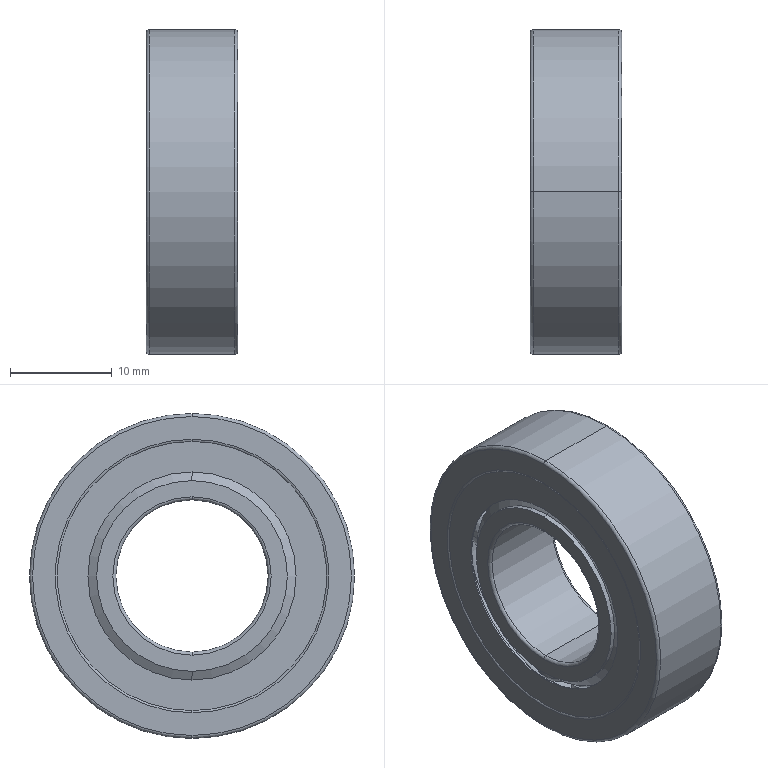Part | SolidWorks | features Revolution 5, CirPattern 2, RefAxis 1, RevCut 1 | 16 solids | 192 faces | box 9 x 32 x 32 mm | volume 4173 mm3 | cylinder 70 | sphere 60 | plane 36 | torus 22 | cone 4 | commonest cylinder face diameters 22.65 x27 24.35 x27 18.778 x4 20.667 x4 26.333 x4 15 x2